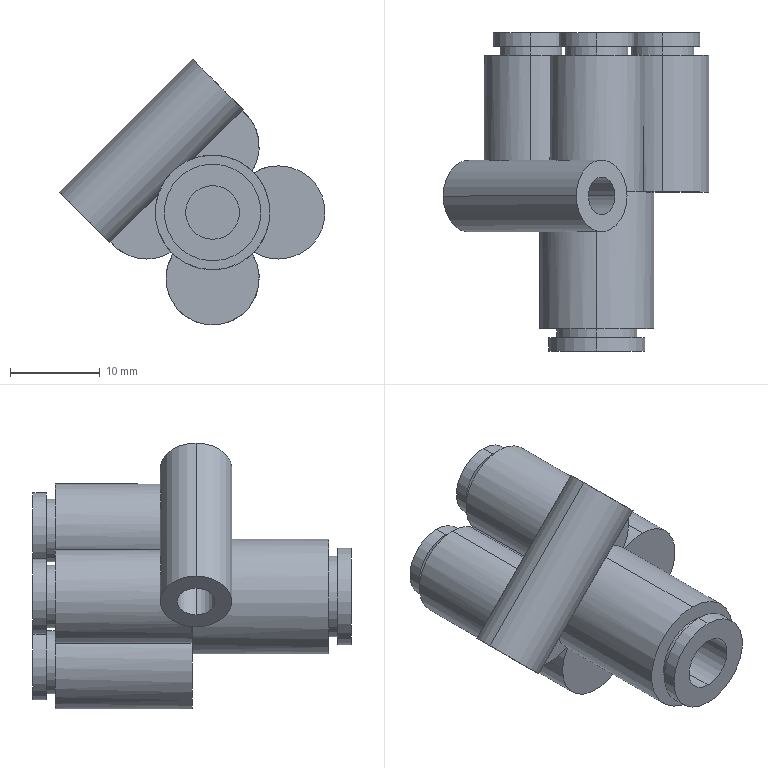Part | SolidWorks | features BaseBody 1 | 1 solid | 102 faces | box 29.666 x 35.5 x 29.666 mm | volume 7119 mm3 | cylinder 60 | plane 40 | spline 2 | commonest cylinder face diameters 10.4 x14 2 x8 4 x8 7 x8 8.4 x8 8 x4